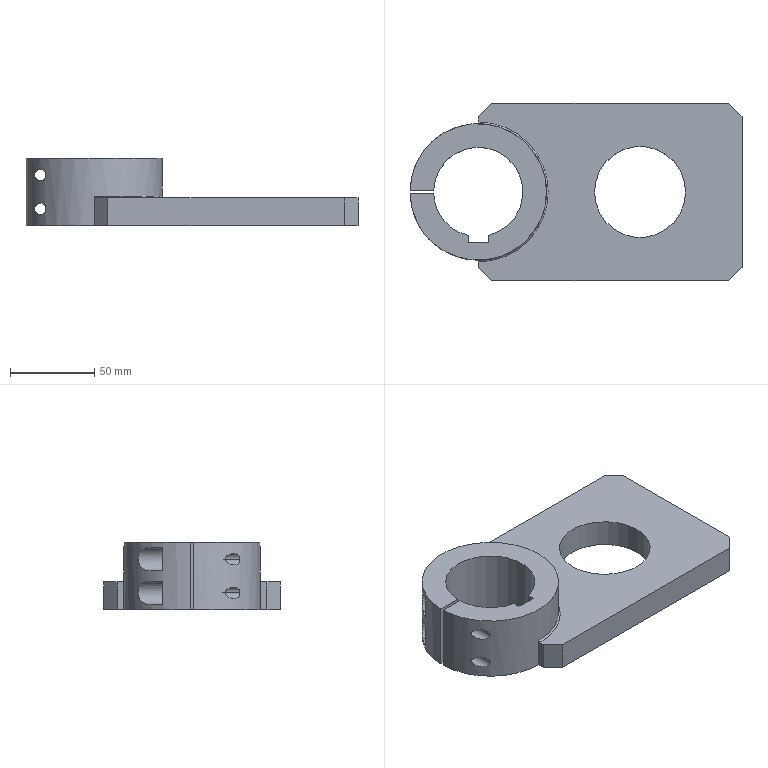Part | Creo | features CURVE 4, CUT 3, DATUM PLANE 3, CHAMFER 1, COORDINATE SYSTEM 1, PROTRUSION 1 | 1 solid | 42 faces | box 196.988 x 105 x 40 mm | volume 298699 mm3 | plane 26 | cylinder 15 | cone 1 | commonest cylinder face diameters 6.8 x8 14 x2 53 x2 54 x2 81 x1
STEP:
#1=CARTESIAN_POINT('',(0.,0.,0.));
#2=DIRECTION('',(0.,0.,1.));
#3=DIRECTION('',(1.,0.,0.));
#4=AXIS2_PLACEMENT_3D('',#1,#2,#3);
#5=CARTESIAN_POINT('',(-40.,44.5,0.));
#6=VERTEX_POINT('',#5);
#7=CARTESIAN_POINT('',(-40.,40.5,0.));
#8=VERTEX_POINT('',#7);
#9=CARTESIAN_POINT('',(-40.,44.5,0.));
#10=DIRECTION('',(0.,-1.,0.));
#11=VECTOR('',#10,4.);
#12=LINE('',#9,#11);
#13=EDGE_CURVE('',#6,#8,#12,.T.);
#14=ORIENTED_EDGE('',*,*,#13,.T.);
#15=CARTESIAN_POINT('',(-80.488,1.,0.));
#16=VERTEX_POINT('',#15);
#17=CARTESIAN_POINT('',(-40.,0.,0.));
#18=DIRECTION('',(0.,0.,1.));
#19=DIRECTION('',(0.,1.,0.));
#20=AXIS2_PLACEMENT_3D('',#17,#18,#19);
#21=CIRCLE('',#20,40.5);
#22=EDGE_CURVE('',#8,#16,#21,.T.);
#23=ORIENTED_EDGE('',*,*,#22,.T.);
#24=CARTESIAN_POINT('',(-66.481,1.,0.));
#25=VERTEX_POINT('',#24);
#26=CARTESIAN_POINT('',(-80.488,1.,0.));
#27=DIRECTION('',(1.,0.,0.));
#28=VECTOR('',#27,14.007);
#29=LINE('',#26,#28);
#30=EDGE_CURVE('',#16,#25,#29,.T.);
#31=ORIENTED_EDGE('',*,*,#30,.T.);
#32=CARTESIAN_POINT('',(-34.,-25.812,0.));
#33=VERTEX_POINT('',#32);
#34=CARTESIAN_POINT('',(-40.,0.,0.));
#35=DIRECTION('',(0.,0.,-1.));
#36=DIRECTION('',(-0.9993,0.03774,0.));
#37=AXIS2_PLACEMENT_3D('',#34,#35,#36);
#38=CIRCLE('',#37,26.5);
#39=EDGE_CURVE('',#25,#33,#38,.T.);
#40=ORIENTED_EDGE('',*,*,#39,.T.);
#41=CARTESIAN_POINT('',(-34.,-30.,0.));
#42=VERTEX_POINT('',#41);
#43=CARTESIAN_POINT('',(-34.,-25.812,0.));
#44=DIRECTION('',(0.,-1.,0.));
#45=VECTOR('',#44,4.188);
#46=LINE('',#43,#45);
#47=EDGE_CURVE('',#33,#42,#46,.T.);
#48=ORIENTED_EDGE('',*,*,#47,.T.);
#49=CARTESIAN_POINT('',(-40.,-30.,0.));
#50=VERTEX_POINT('',#49);
#51=CARTESIAN_POINT('',(-34.,-30.,0.));
#52=DIRECTION('',(-1.,0.,0.));
#53=VECTOR('',#52,6.);
#54=LINE('',#51,#53);
#55=EDGE_CURVE('',#42,#50,#54,.T.);
#56=ORIENTED_EDGE('',*,*,#55,.T.);
#57=CARTESIAN_POINT('',(-46.,-30.,0.));
#58=VERTEX_POINT('',#57);
#59=CARTESIAN_POINT('',(-40.,-30.,0.));
#60=DIRECTION('',(-1.,0.,0.));
#61=VECTOR('',#60,6.);
#62=LINE('',#59,#61);
#63=EDGE_CURVE('',#50,#58,#62,.T.);
#64=ORIENTED_EDGE('',*,*,#63,.T.);
#65=CARTESIAN_POINT('',(-46.,-25.812,0.));
#66=VERTEX_POINT('',#65);
#67=CARTESIAN_POINT('',(-46.,-30.,0.));
#68=DIRECTION('',(0.,1.,0.));
#69=VECTOR('',#68,4.188);
#70=LINE('',#67,#69);
#71=EDGE_CURVE('',#58,#66,#70,.T.);
#72=ORIENTED_EDGE('',*,*,#71,.T.);
#73=CARTESIAN_POINT('',(-66.481,-1.,0.));
#74=VERTEX_POINT('',#73);
#75=CARTESIAN_POINT('',(-40.,0.,0.));
#76=DIRECTION('',(0.,0.,-1.));
#77=DIRECTION('',(-0.2264,-0.974,0.));
#78=AXIS2_PLACEMENT_3D('',#75,#76,#77);
#79=CIRCLE('',#78,26.5);
#80=EDGE_CURVE('',#66,#74,#79,.T.);
#81=ORIENTED_EDGE('',*,*,#80,.T.);
#82=CARTESIAN_POINT('',(-80.488,-1.,0.));
#83=VERTEX_POINT('',#82);
#84=CARTESIAN_POINT('',(-66.481,-1.,0.));
#85=DIRECTION('',(-1.,0.,0.));
#86=VECTOR('',#85,14.007);
#87=LINE('',#84,#86);
#88=EDGE_CURVE('',#74,#83,#87,.T.);
#89=ORIENTED_EDGE('',*,*,#88,.T.);
#90=CARTESIAN_POINT('',(-40.,-40.5,0.));
#91=VERTEX_POINT('',#90);
#92=CARTESIAN_POINT('',(-40.,0.,0.));
#93=DIRECTION('',(0.,0.,1.));
#94=DIRECTION('',(-0.9997,-0.02469,0.));
#95=AXIS2_PLACEMENT_3D('',#92,#93,#94);
#96=CIRCLE('',#95,40.5);
#97=EDGE_CURVE('',#83,#91,#96,.T.);
#98=ORIENTED_EDGE('',*,*,#97,.T.);
#99=CARTESIAN_POINT('',(-40.,-44.5,0.));
#100=VERTEX_POINT('',#99);
#101=CARTESIAN_POINT('',(-40.,-40.5,0.));
#102=DIRECTION('',(0.,-1.,0.));
#103=VECTOR('',#102,4.);
#104=LINE('',#101,#103);
#105=EDGE_CURVE('',#91,#100,#104,.T.);
#106=ORIENTED_EDGE('',*,*,#105,.T.);
#107=CARTESIAN_POINT('',(-32.,-52.5,0.));
#108=VERTEX_POINT('',#107);
#109=CARTESIAN_POINT('',(-40.,-44.5,0.));
#110=DIRECTION('',(0.7071,-0.7071,0.));
#111=VECTOR('',#110,11.314);
#112=LINE('',#109,#111);
#113=EDGE_CURVE('',#100,#108,#112,.T.);
#114=ORIENTED_EDGE('',*,*,#113,.T.);
#115=CARTESIAN_POINT('',(108.5,-52.5,0.));
#116=VERTEX_POINT('',#115);
#117=CARTESIAN_POINT('',(-32.,-52.5,0.));
#118=DIRECTION('',(1.,0.,0.));
#119=VECTOR('',#118,140.5);
#120=LINE('',#117,#119);
#121=EDGE_CURVE('',#108,#116,#120,.T.);
#122=ORIENTED_EDGE('',*,*,#121,.T.);
#123=CARTESIAN_POINT('',(116.5,-44.5,0.));
#124=VERTEX_POINT('',#123);
#125=CARTESIAN_POINT('',(108.5,-52.5,0.));
#126=DIRECTION('',(0.7071,0.7071,0.));
#127=VECTOR('',#126,11.314);
#128=LINE('',#125,#127);
#129=EDGE_CURVE('',#116,#124,#128,.T.);
#130=ORIENTED_EDGE('',*,*,#129,.T.);
#131=CARTESIAN_POINT('',(116.5,44.5,0.));
#132=VERTEX_POINT('',#131);
#133=CARTESIAN_POINT('',(116.5,-44.5,0.));
#134=DIRECTION('',(0.,1.,0.));
#135=VECTOR('',#134,89.);
#136=LINE('',#133,#135);
#137=EDGE_CURVE('',#124,#132,#136,.T.);
#138=ORIENTED_EDGE('',*,*,#137,.T.);
#139=CARTESIAN_POINT('',(108.5,52.5,0.));
#140=VERTEX_POINT('',#139);
#141=CARTESIAN_POINT('',(116.5,44.5,0.));
#142=DIRECTION('',(-0.7071,0.7071,0.));
#143=VECTOR('',#142,11.314);
#144=LINE('',#141,#143);
#145=EDGE_CURVE('',#132,#140,#144,.T.);
#146=ORIENTED_EDGE('',*,*,#145,.T.);
#147=CARTESIAN_POINT('',(-32.,52.5,0.));
#148=VERTEX_POINT('',#147);
#149=CARTESIAN_POINT('',(108.5,52.5,0.));
#150=DIRECTION('',(-1.,0.,0.));
#151=VECTOR('',#150,140.5);
#152=LINE('',#149,#151);
#153=EDGE_CURVE('',#140,#148,#152,.T.);
#154=ORIENTED_EDGE('',*,*,#153,.T.);
#155=CARTESIAN_POINT('',(-32.,52.5,0.));
#156=DIRECTION('',(-0.7071,-0.7071,0.));
#157=VECTOR('',#156,11.314);
#158=LINE('',#155,#157);
#159=EDGE_CURVE('',#148,#6,#158,.T.);
#160=ORIENTED_EDGE('',*,*,#159,.T.);
#161=EDGE_LOOP('',(#14,#23,#31,#40,#48,#56,#64,#72,#81,#89,#98,#106,#114,#122,#130,#138,#146,#154,#160));
#162=FACE_OUTER_BOUND('',#161,.F.);
#163=CARTESIAN_POINT('',(83.,0.,0.));
#164=VERTEX_POINT('',#163);
#165=CARTESIAN_POINT('',(29.,0.,0.));
#166=VERTEX_POINT('',#165);
#167=CARTESIAN_POINT('',(56.,0.,0.));
#168=DIRECTION('',(0.,0.,-1.));
#169=DIRECTION('',(1.,0.,0.));
#170=AXIS2_PLACEMENT_3D('',#167,#168,#169);
#171=CIRCLE('',#170,27.);
#172=EDGE_CURVE('',#164,#166,#171,.T.);
#173=ORIENTED_EDGE('',*,*,#172,.T.);
#174=CARTESIAN_POINT('',(56.,0.,0.));
#175=DIRECTION('',(0.,0.,-1.));
#176=DIRECTION('',(-1.,0.,0.));
#177=AXIS2_PLACEMENT_3D('',#174,#175,#176);
#178=CIRCLE('',#177,27.);
#179=EDGE_CURVE('',#166,#164,#178,.T.);
#180=ORIENTED_EDGE('',*,*,#179,.T.);
#181=EDGE_LOOP('',(#173,#180));
#182=FACE_BOUND('',#181,.F.);
#183=CARTESIAN_POINT('',(0.,0.,0.));
#184=DIRECTION('',(0.,0.,1.));
#185=DIRECTION('',(1.,0.,0.));
#186=AXIS2_PLACEMENT_3D('',#183,#184,#185);
#187=PLANE('',#186);
#188=ADVANCED_FACE('',(#162,#182),#187,.F.);
#189=CARTESIAN_POINT('',(29.,0.,16.5));
#190=VERTEX_POINT('',#189);
#191=CARTESIAN_POINT('',(83.,0.,16.5));
#192=VERTEX_POINT('',#191);
#193=CARTESIAN_POINT('',(56.,0.,16.5));
#194=DIRECTION('',(0.,0.,1.));
#195=DIRECTION('',(-1.,0.,0.));
#196=AXIS2_PLACEMENT_3D('',#193,#194,#195);
#197=CIRCLE('',#196,27.);
#198=EDGE_CURVE('',#190,#192,#197,.T.);
#199=ORIENTED_EDGE('',*,*,#198,.F.);
#200=CARTESIAN_POINT('',(29.,0.,0.));
#201=DIRECTION('',(0.,0.,1.));
#202=VECTOR('',#201,16.5);
#203=LINE('',#200,#202);
#204=EDGE_CURVE('',#166,#190,#203,.T.);
#205=ORIENTED_EDGE('',*,*,#204,.F.);
#206=ORIENTED_EDGE('',*,*,#172,.F.);
#207=CARTESIAN_POINT('',(83.,0.,0.));
#208=DIRECTION('',(0.,0.,1.));
#209=VECTOR('',#208,16.5);
#210=LINE('',#207,#209);
#211=EDGE_CURVE('',#164,#192,#210,.T.);
#212=ORIENTED_EDGE('',*,*,#211,.T.);
#213=EDGE_LOOP('',(#199,#205,#206,#212));
#214=FACE_OUTER_BOUND('',#213,.F.);
#215=CARTESIAN_POINT('',(56.,0.,0.));
#216=DIRECTION('',(0.,0.,1.));
#217=DIRECTION('',(1.,0.,0.));
#218=AXIS2_PLACEMENT_3D('',#215,#216,#217);
#219=CYLINDRICAL_SURFACE('',#218,27.);
#220=ADVANCED_FACE('',(#214),#219,.F.);
#221=CARTESIAN_POINT('',(-40.,41.5,16.5));
#222=VERTEX_POINT('',#221);
#223=CARTESIAN_POINT('',(-40.,-41.5,16.5));
#224=VERTEX_POINT('',#223);
#225=CARTESIAN_POINT('',(-40.,0.000000008,16.5));
#226=DIRECTION('',(0.,0.,-1.));
#227=DIRECTION('',(0.,1.,0.));
#228=AXIS2_PLACEMENT_3D('',#225,#226,#227);
#229=CIRCLE('',#228,41.5);
#230=EDGE_CURVE('',#222,#224,#229,.T.);
#231=ORIENTED_EDGE('',*,*,#230,.F.);
#232=CARTESIAN_POINT('',(-40.,44.5,16.5));
#233=VERTEX_POINT('',#232);
#234=CARTESIAN_POINT('',(-40.,44.5,16.5));
#235=DIRECTION('',(0.,-1.,0.000000001));
#236=VECTOR('',#235,3.);
#237=LINE('',#234,#236);
#238=EDGE_CURVE('',#233,#222,#237,.T.);
#239=ORIENTED_EDGE('',*,*,#238,.F.);
#240=CARTESIAN_POINT('',(-32.,52.5,16.5));
#241=VERTEX_POINT('',#240);
#242=CARTESIAN_POINT('',(-32.,52.5,16.5));
#243=DIRECTION('',(-0.7071,-0.7071,0.));
#244=VECTOR('',#243,11.314);
#245=LINE('',#242,#244);
#246=EDGE_CURVE('',#241,#233,#245,.T.);
#247=ORIENTED_EDGE('',*,*,#246,.F.);
#248=CARTESIAN_POINT('',(108.5,52.5,16.5));
#249=VERTEX_POINT('',#248);
#250=CARTESIAN_POINT('',(108.5,52.5,16.5));
#251=DIRECTION('',(-1.,0.,0.));
#252=VECTOR('',#251,140.5);
#253=LINE('',#250,#252);
#254=EDGE_CURVE('',#249,#241,#253,.T.);
#255=ORIENTED_EDGE('',*,*,#254,.F.);
#256=CARTESIAN_POINT('',(116.5,44.5,16.5));
#257=VERTEX_POINT('',#256);
#258=CARTESIAN_POINT('',(116.5,44.5,16.5));
#259=DIRECTION('',(-0.7071,0.7071,0.));
#260=VECTOR('',#259,11.314);
#261=LINE('',#258,#260);
#262=EDGE_CURVE('',#257,#249,#261,.T.);
#263=ORIENTED_EDGE('',*,*,#262,.F.);
#264=CARTESIAN_POINT('',(116.5,-44.5,16.5));
#265=VERTEX_POINT('',#264);
#266=CARTESIAN_POINT('',(116.5,-44.5,16.5));
#267=DIRECTION('',(0.,1.,0.));
#268=VECTOR('',#267,89.);
#269=LINE('',#266,#268);
#270=EDGE_CURVE('',#265,#257,#269,.T.);
#271=ORIENTED_EDGE('',*,*,#270,.F.);
#272=CARTESIAN_POINT('',(108.5,-52.5,16.5));
#273=VERTEX_POINT('',#272);
#274=CARTESIAN_POINT('',(108.5,-52.5,16.5));
#275=DIRECTION('',(0.7071,0.7071,0.));
#276=VECTOR('',#275,11.314);
#277=LINE('',#274,#276);
#278=EDGE_CURVE('',#273,#265,#277,.T.);
#279=ORIENTED_EDGE('',*,*,#278,.F.);
#280=CARTESIAN_POINT('',(-32.,-52.5,16.5));
#281=VERTEX_POINT('',#280);
#282=CARTESIAN_POINT('',(-32.,-52.5,16.5));
#283=DIRECTION('',(1.,0.,0.));
#284=VECTOR('',#283,140.5);
#285=LINE('',#282,#284);
#286=EDGE_CURVE('',#281,#273,#285,.T.);
#287=ORIENTED_EDGE('',*,*,#286,.F.);
#288=CARTESIAN_POINT('',(-40.,-44.5,16.5));
#289=VERTEX_POINT('',#288);
#290=CARTESIAN_POINT('',(-40.,-44.5,16.5));
#291=DIRECTION('',(0.7071,-0.7071,0.));
#292=VECTOR('',#291,11.314);
#293=LINE('',#290,#292);
#294=EDGE_CURVE('',#289,#281,#293,.T.);
#295=ORIENTED_EDGE('',*,*,#294,.F.);
#296=CARTESIAN_POINT('',(-40.,-41.5,16.5));
#297=DIRECTION('',(0.,-1.,0.));
#298=VECTOR('',#297,3.);
#299=LINE('',#296,#298);
#300=EDGE_CURVE('',#224,#289,#299,.T.);
#301=ORIENTED_EDGE('',*,*,#300,.F.);
#302=EDGE_LOOP('',(#231,#239,#247,#255,#263,#271,#279,#287,#295,#301));
#303=FACE_OUTER_BOUND('',#302,.F.);
#304=ORIENTED_EDGE('',*,*,#198,.T.);
#305=CARTESIAN_POINT('',(56.,0.,16.5));
#306=DIRECTION('',(0.,0.,1.));
#307=DIRECTION('',(1.,0.,0.));
#308=AXIS2_PLACEMENT_3D('',#305,#306,#307);
#309=CIRCLE('',#308,27.);
#310=EDGE_CURVE('',#192,#190,#309,.T.);
#311=ORIENTED_EDGE('',*,*,#310,.T.);
#312=EDGE_LOOP('',(#304,#311));
#313=FACE_BOUND('',#312,.F.);
#314=CARTESIAN_POINT('',(0.,0.,16.5));
#315=DIRECTION('',(0.,0.,1.));
#316=DIRECTION('',(1.,0.,0.));
#317=AXIS2_PLACEMENT_3D('',#314,#315,#316);
#318=PLANE('',#317);
#319=ADVANCED_FACE('',(#303,#313),#318,.T.);
#320=ORIENTED_EDGE('',*,*,#310,.F.);
#321=ORIENTED_EDGE('',*,*,#211,.F.);
#322=ORIENTED_EDGE('',*,*,#179,.F.);
#323=ORIENTED_EDGE('',*,*,#204,.T.);
#324=EDGE_LOOP('',(#320,#321,#322,#323));
#325=FACE_OUTER_BOUND('',#324,.F.);
#326=CARTESIAN_POINT('',(56.,0.,0.));
#327=DIRECTION('',(0.,0.,1.));
#328=DIRECTION('',(1.,0.,0.));
#329=AXIS2_PLACEMENT_3D('',#326,#327,#328);
#330=CYLINDRICAL_SURFACE('',#329,27.);
#331=ADVANCED_FACE('',(#325),#330,.F.);
#332=CARTESIAN_POINT('',(-40.,-40.5,17.5));
#333=VERTEX_POINT('',#332);
#334=CARTESIAN_POINT('',(-40.,40.5,17.5));
#335=VERTEX_POINT('',#334);
#336=CARTESIAN_POINT('',(-40.,0.000000008,17.5));
#337=DIRECTION('',(0.,0.,1.));
#338=DIRECTION('',(0.,-1.,0.));
#339=AXIS2_PLACEMENT_3D('',#336,#337,#338);
#340=CIRCLE('',#339,40.5);
#341=EDGE_CURVE('',#333,#335,#340,.T.);
#342=ORIENTED_EDGE('',*,*,#341,.T.);
#343=CARTESIAN_POINT('',(-40.,40.5,17.5));
#344=DIRECTION('',(0.,0.7071,-0.7071));
#345=VECTOR('',#344,1.414);
#346=LINE('',#343,#345);
#347=EDGE_CURVE('',#335,#222,#346,.T.);
#348=ORIENTED_EDGE('',*,*,#347,.T.);
#349=ORIENTED_EDGE('',*,*,#230,.T.);
#350=CARTESIAN_POINT('',(-40.,-41.5,16.5));
#351=DIRECTION('',(0.,0.7071,0.7071));
#352=VECTOR('',#351,1.414);
#353=LINE('',#350,#352);
#354=EDGE_CURVE('',#224,#333,#353,.T.);
#355=ORIENTED_EDGE('',*,*,#354,.T.);
#356=EDGE_LOOP('',(#342,#348,#349,#355));
#357=FACE_OUTER_BOUND('',#356,.F.);
#358=CARTESIAN_POINT('',(-40.,0.000000008,17.));
#359=DIRECTION('',(0.,0.,-1.));
#360=DIRECTION('',(0.,-1.,0.));
#361=AXIS2_PLACEMENT_3D('',#358,#359,#360);
#362=CONICAL_SURFACE('',#361,41.,45.);
#363=ADVANCED_FACE('',(#357),#362,.T.);
#364=ORIENTED_EDGE('',*,*,#341,.F.);
#365=CARTESIAN_POINT('',(-40.,-40.5,0.));
#366=DIRECTION('',(0.,0.,1.));
#367=VECTOR('',#366,17.5);
#368=LINE('',#365,#367);
#369=EDGE_CURVE('',#91,#333,#368,.T.);
#370=ORIENTED_EDGE('',*,*,#369,.F.);
#371=ORIENTED_EDGE('',*,*,#97,.F.);
#372=CARTESIAN_POINT('',(-80.488,-1.,40.));
#373=VERTEX_POINT('',#372);
#374=CARTESIAN_POINT('',(-80.488,-1.,0.));
#375=DIRECTION('',(0.,0.,1.));
#376=VECTOR('',#375,40.);
#377=LINE('',#374,#376);
#378=EDGE_CURVE('',#83,#373,#377,.T.);
#379=ORIENTED_EDGE('',*,*,#378,.T.);
#380=CARTESIAN_POINT('',(-80.488,1.,40.));
#381=VERTEX_POINT('',#380);
#382=CARTESIAN_POINT('',(-40.,0.,40.));
#383=DIRECTION('',(0.,0.,1.));
#384=DIRECTION('',(-0.9997,-0.02469,0.));
#385=AXIS2_PLACEMENT_3D('',#382,#383,#384);
#386=CIRCLE('',#385,40.5);
#387=EDGE_CURVE('',#373,#381,#386,.T.);
#388=ORIENTED_EDGE('',*,*,#387,.T.);
#389=CARTESIAN_POINT('',(-80.488,1.,0.));
#390=DIRECTION('',(0.,0.,1.));
#391=VECTOR('',#390,40.);
#392=LINE('',#389,#391);
#393=EDGE_CURVE('',#16,#381,#392,.T.);
#394=ORIENTED_EDGE('',*,*,#393,.F.);
#395=ORIENTED_EDGE('',*,*,#22,.F.);
#396=CARTESIAN_POINT('',(-40.,40.5,17.5));
#397=DIRECTION('',(0.,0.,-1.));
#398=VECTOR('',#397,17.5);
#399=LINE('',#396,#398);
#400=EDGE_CURVE('',#335,#8,#399,.T.);
#401=ORIENTED_EDGE('',*,*,#400,.F.);
#402=EDGE_LOOP('',(#364,#370,#371,#379,#388,#394,#395,#401));
#403=FACE_OUTER_BOUND('',#402,.F.);
#404=CARTESIAN_POINT('',(-68.923,-28.35,8.554));
#405=VERTEX_POINT('',#404);
#406=CARTESIAN_POINT('',(-68.923,-28.35,11.446));
#407=VERTEX_POINT('',#406);
#408=CARTESIAN_POINT('',(-68.923,-28.35,8.554));
#409=DIRECTION('',(0.,0.,1.));
#410=VECTOR('',#409,2.892);
#411=LINE('',#408,#410);
#412=EDGE_CURVE('',#405,#407,#411,.T.);
#413=ORIENTED_EDGE('',*,*,#412,.T.);
#414=CARTESIAN_POINT('',(-75.4,-19.675,10.));
#415=VERTEX_POINT('',#414);
#416=CARTESIAN_POINT('',(-75.4,-19.675,10.194));
#417=CARTESIAN_POINT('',(-75.368,-19.733,10.574));
#418=CARTESIAN_POINT('',(-75.223,-19.992,11.133));
#419=CARTESIAN_POINT('',(-74.989,-20.398,11.652));
#420=CARTESIAN_POINT('',(-74.679,-20.922,12.118));
#421=CARTESIAN_POINT('',(-74.297,-21.544,12.528));
#422=CARTESIAN_POINT('',(-73.838,-22.26,12.88));
#423=CARTESIAN_POINT('',(-73.311,-23.043,13.157));
#424=CARTESIAN_POINT('',(-72.705,-23.897,13.348));
#425=CARTESIAN_POINT('',(-72.034,-24.789,13.423));
#426=CARTESIAN_POINT('',(-71.32,-25.686,13.359));
#427=CARTESIAN_POINT('',(-70.573,-26.57,13.122));
#428=CARTESIAN_POINT('',(-69.869,-27.357,12.69));
#429=CARTESIAN_POINT('',(-69.31,-27.952,12.128));
#430=CARTESIAN_POINT('',(-69.035,-28.235,11.685));
#431=CARTESIAN_POINT('',(-68.923,-28.35,11.446));
#432=B_SPLINE_CURVE_WITH_KNOTS('',3,(#414,#416,#417,#418,#419,#420,#421,#422,#423,#424,#425,#426,#427,#428,#429,#430,#431),.UNSPECIFIED.,.F.,.F.,(4,1,1,1,1,1,1,1,1,1,1,1,1,1,4),(0.,0.07143,0.1429,0.2143,0.2857,0.3571,0.4286,0.5,0.5714,0.6429,0.7143,0.7857,0.8571,0.9286,1.),.UNSPECIFIED.);
#433=EDGE_CURVE('',#415,#407,#432,.T.);
#434=ORIENTED_EDGE('',*,*,#433,.F.);
#435=CARTESIAN_POINT('',(-68.923,-28.35,8.554));
#436=CARTESIAN_POINT('',(-69.044,-28.226,8.296));
#437=CARTESIAN_POINT('',(-69.345,-27.916,7.819));
#438=CARTESIAN_POINT('',(-69.987,-27.23,7.211));
#439=CARTESIAN_POINT('',(-70.781,-26.331,6.786));
#440=CARTESIAN_POINT('',(-71.589,-25.356,6.595));
#441=CARTESIAN_POINT('',(-72.34,-24.39,6.591));
#442=CARTESIAN_POINT('',(-73.025,-23.452,6.735));
#443=CARTESIAN_POINT('',(-73.627,-22.579,6.992));
#444=CARTESIAN_POINT('',(-74.14,-21.795,7.334));
#445=CARTESIAN_POINT('',(-74.579,-21.089,7.757));
#446=CARTESIAN_POINT('',(-74.931,-20.499,8.243));
#447=CARTESIAN_POINT('',(-75.192,-20.045,8.778));
#448=CARTESIAN_POINT('',(-75.361,-19.745,9.375));
#449=CARTESIAN_POINT('',(-75.4,-19.675,9.788));
#450=CARTESIAN_POINT('',(-75.4,-19.675,10.));
#451=B_SPLINE_CURVE_WITH_KNOTS('',3,(#435,#436,#437,#438,#439,#440,#441,#442,#443,#444,#445,#446,#447,#448,#449,#450),.UNSPECIFIED.,.F.,.F.,(4,1,1,1,1,1,1,1,1,1,1,1,1,4),(0.,0.07692,0.1538,0.2308,0.3077,0.3846,0.4615,0.5385,0.6154,0.6923,0.7692,0.8462,0.9231,1.),.UNSPECIFIED.);
#452=EDGE_CURVE('',#405,#415,#451,.T.);
#453=ORIENTED_EDGE('',*,*,#452,.F.);
#454=EDGE_LOOP('',(#413,#434,#453));
#455=FACE_BOUND('',#454,.F.);
#456=CARTESIAN_POINT('',(-68.923,-28.35,28.554));
#457=VERTEX_POINT('',#456);
#458=CARTESIAN_POINT('',(-68.923,-28.35,31.446));
#459=VERTEX_POINT('',#458);
#460=CARTESIAN_POINT('',(-68.923,-28.35,28.554));
#461=DIRECTION('',(0.,0.,1.));
#462=VECTOR('',#461,2.892);
#463=LINE('',#460,#462);
#464=EDGE_CURVE('',#457,#459,#463,.T.);
#465=ORIENTED_EDGE('',*,*,#464,.T.);
#466=CARTESIAN_POINT('',(-75.4,-19.675,30.));
#467=VERTEX_POINT('',#466);
#468=CARTESIAN_POINT('',(-75.4,-19.675,30.194));
#469=CARTESIAN_POINT('',(-75.368,-19.733,30.574));
#470=CARTESIAN_POINT('',(-75.223,-19.992,31.133));
#471=CARTESIAN_POINT('',(-74.989,-20.398,31.652));
#472=CARTESIAN_POINT('',(-74.679,-20.922,32.118));
#473=CARTESIAN_POINT('',(-74.297,-21.544,32.528));
#474=CARTESIAN_POINT('',(-73.838,-22.26,32.88));
#475=CARTESIAN_POINT('',(-73.311,-23.043,33.157));
#476=CARTESIAN_POINT('',(-72.705,-23.897,33.348));
#477=CARTESIAN_POINT('',(-72.034,-24.789,33.423));
#478=CARTESIAN_POINT('',(-71.32,-25.686,33.359));
#479=CARTESIAN_POINT('',(-70.573,-26.57,33.122));
#480=CARTESIAN_POINT('',(-69.869,-27.357,32.69));
#481=CARTESIAN_POINT('',(-69.31,-27.952,32.128));
#482=CARTESIAN_POINT('',(-69.035,-28.235,31.685));
#483=CARTESIAN_POINT('',(-68.923,-28.35,31.446));
#484=B_SPLINE_CURVE_WITH_KNOTS('',3,(#466,#468,#469,#470,#471,#472,#473,#474,#475,#476,#477,#478,#479,#480,#481,#482,#483),.UNSPECIFIED.,.F.,.F.,(4,1,1,1,1,1,1,1,1,1,1,1,1,1,4),(0.,0.07143,0.1429,0.2143,0.2857,0.3571,0.4286,0.5,0.5714,0.6429,0.7143,0.7857,0.8571,0.9286,1.),.UNSPECIFIED.);
#485=EDGE_CURVE('',#467,#459,#484,.T.);
#486=ORIENTED_EDGE('',*,*,#485,.F.);
#487=CARTESIAN_POINT('',(-68.923,-28.35,28.554));
#488=CARTESIAN_POINT('',(-69.044,-28.226,28.296));
#489=CARTESIAN_POINT('',(-69.345,-27.916,27.819));
#490=CARTESIAN_POINT('',(-69.987,-27.23,27.211));
#491=CARTESIAN_POINT('',(-70.781,-26.331,26.786));
#492=CARTESIAN_POINT('',(-71.589,-25.356,26.595));
#493=CARTESIAN_POINT('',(-72.34,-24.39,26.591));
#494=CARTESIAN_POINT('',(-73.025,-23.452,26.735));
#495=CARTESIAN_POINT('',(-73.627,-22.579,26.992));
#496=CARTESIAN_POINT('',(-74.14,-21.795,27.334));
#497=CARTESIAN_POINT('',(-74.579,-21.089,27.757));
#498=CARTESIAN_POINT('',(-74.931,-20.499,28.243));
#499=CARTESIAN_POINT('',(-75.192,-20.045,28.778));
#500=CARTESIAN_POINT('',(-75.361,-19.745,29.375));
#501=CARTESIAN_POINT('',(-75.4,-19.675,29.788));
#502=CARTESIAN_POINT('',(-75.4,-19.675,30.));
#503=B_SPLINE_CURVE_WITH_KNOTS('',3,(#487,#488,#489,#490,#491,#492,#493,#494,#495,#496,#497,#498,#499,#500,#501,#502),.UNSPECIFIED.,.F.,.F.,(4,1,1,1,1,1,1,1,1,1,1,1,1,4),(0.,0.07692,0.1538,0.2308,0.3077,0.3846,0.4615,0.5385,0.6154,0.6923,0.7692,0.8462,0.9231,1.),.UNSPECIFIED.);
#504=EDGE_CURVE('',#457,#467,#503,.T.);
#505=ORIENTED_EDGE('',*,*,#504,.F.);
#506=EDGE_LOOP('',(#465,#486,#505));
#507=FACE_BOUND('',#506,.F.);
#508=CARTESIAN_POINT('',(-76.524,17.5,3.));
#509=VERTEX_POINT('',#508);
#510=CARTESIAN_POINT('',(-76.524,17.5,17.));
#511=VERTEX_POINT('',#510);
#512=CARTESIAN_POINT('',(-76.524,17.5,3.));
#513=DIRECTION('',(0.,0.,1.));
#514=VECTOR('',#513,14.);
#515=LINE('',#512,#514);
#516=EDGE_CURVE('',#509,#511,#515,.T.);
#517=ORIENTED_EDGE('',*,*,#516,.T.);
#518=CARTESIAN_POINT('',(-72.,24.824,17.));
#519=VERTEX_POINT('',#518);
#520=CARTESIAN_POINT('',(-40.,0.,17.));
#521=DIRECTION('',(0.,0.,1.));
#522=DIRECTION('',(-0.7901,0.6129,0.));
#523=AXIS2_PLACEMENT_3D('',#520,#521,#522);
#524=CIRCLE('',#523,40.5);
#525=EDGE_CURVE('',#519,#511,#524,.T.);
#526=ORIENTED_EDGE('',*,*,#525,.F.);
#527=CARTESIAN_POINT('',(-72.,24.824,3.));
#528=VERTEX_POINT('',#527);
#529=CARTESIAN_POINT('',(-71.732,25.17,3.));
#530=CARTESIAN_POINT('',(-71.187,25.849,3.031));
#531=CARTESIAN_POINT('',(-70.34,26.839,3.181));
#532=CARTESIAN_POINT('',(-69.473,27.787,3.45));
#533=CARTESIAN_POINT('',(-68.599,28.685,3.855));
#534=CARTESIAN_POINT('',(-67.74,29.516,4.412));
#535=CARTESIAN_POINT('',(-66.929,30.256,5.131));
#536=CARTESIAN_POINT('',(-66.195,30.893,6.028));
#537=CARTESIAN_POINT('',(-65.577,31.405,7.117));
#538=CARTESIAN_POINT('',(-65.132,31.76,8.417));
#539=CARTESIAN_POINT('',(-64.952,31.901,9.857));
#540=CARTESIAN_POINT('',(-65.07,31.809,11.283));
#541=CARTESIAN_POINT('',(-65.464,31.495,12.623));
#542=CARTESIAN_POINT('',(-66.046,31.018,13.748));
#543=CARTESIAN_POINT('',(-66.774,30.394,14.705));
#544=CARTESIAN_POINT('',(-67.593,29.653,15.476));
#545=CARTESIAN_POINT('',(-68.484,28.8,16.083));
#546=CARTESIAN_POINT('',(-69.391,27.875,16.52));
#547=CARTESIAN_POINT('',(-70.292,26.894,16.809));
#548=CARTESIAN_POINT('',(-71.168,25.873,16.968));
#549=CARTESIAN_POINT('',(-71.726,25.177,17.));
#550=CARTESIAN_POINT('',(-72.,24.824,17.));
#551=B_SPLINE_CURVE_WITH_KNOTS('',3,(#527,#529,#530,#531,#532,#533,#534,#535,#536,#537,#538,#539,#540,#541,#542,#543,#544,#545,#546,#547,#548,#549,#550),.UNSPECIFIED.,.F.,.F.,(4,1,1,1,1,1,1,1,1,1,1,1,1,1,1,1,1,1,1,1,4),(0.,0.05,0.1,0.15,0.2,0.25,0.3,0.35,0.4,0.45,0.5,0.55,0.6,0.65,0.7,0.75,0.8,0.85,0.9,0.95,1.),.UNSPECIFIED.);
#552=EDGE_CURVE('',#528,#519,#551,.T.);
#553=ORIENTED_EDGE('',*,*,#552,.F.);
#554=CARTESIAN_POINT('',(-40.,0.,3.));
#555=DIRECTION('',(0.,0.,1.));
#556=DIRECTION('',(-0.7901,0.6129,0.));
#557=AXIS2_PLACEMENT_3D('',#554,#555,#556);
#558=CIRCLE('',#557,40.5);
#559=EDGE_CURVE('',#528,#509,#558,.T.);
#560=ORIENTED_EDGE('',*,*,#559,.T.);
#561=EDGE_LOOP('',(#517,#526,#553,#560));
#562=FACE_BOUND('',#561,.F.);
#563=CARTESIAN_POINT('',(-76.524,17.5,23.));
#564=VERTEX_POINT('',#563);
#565=CARTESIAN_POINT('',(-76.524,17.5,37.));
#566=VERTEX_POINT('',#565);
#567=CARTESIAN_POINT('',(-76.524,17.5,23.));
#568=DIRECTION('',(0.,0.,1.));
#569=VECTOR('',#568,14.);
#570=LINE('',#567,#569);
#571=EDGE_CURVE('',#564,#566,#570,.T.);
#572=ORIENTED_EDGE('',*,*,#571,.T.);
#573=CARTESIAN_POINT('',(-72.,24.824,37.));
#574=VERTEX_POINT('',#573);
#575=CARTESIAN_POINT('',(-40.,0.,37.));
#576=DIRECTION('',(0.,0.,1.));
#577=DIRECTION('',(-0.7901,0.6129,0.));
#578=AXIS2_PLACEMENT_3D('',#575,#576,#577);
#579=CIRCLE('',#578,40.5);
#580=EDGE_CURVE('',#574,#566,#579,.T.);
#581=ORIENTED_EDGE('',*,*,#580,.F.);
#582=CARTESIAN_POINT('',(-72.,24.824,23.));
#583=VERTEX_POINT('',#582);
#584=CARTESIAN_POINT('',(-71.732,25.17,23.));
#585=CARTESIAN_POINT('',(-71.187,25.849,23.031));
#586=CARTESIAN_POINT('',(-70.34,26.839,23.181));
#587=CARTESIAN_POINT('',(-69.473,27.787,23.45));
#588=CARTESIAN_POINT('',(-68.599,28.685,23.855));
#589=CARTESIAN_POINT('',(-67.74,29.516,24.412));
#590=CARTESIAN_POINT('',(-66.929,30.256,25.131));
#591=CARTESIAN_POINT('',(-66.195,30.893,26.028));
#592=CARTESIAN_POINT('',(-65.577,31.405,27.117));
#593=CARTESIAN_POINT('',(-65.132,31.76,28.417));
#594=CARTESIAN_POINT('',(-64.952,31.901,29.857));
#595=CARTESIAN_POINT('',(-65.07,31.809,31.283));
#596=CARTESIAN_POINT('',(-65.464,31.495,32.623));
#597=CARTESIAN_POINT('',(-66.046,31.018,33.748));
#598=CARTESIAN_POINT('',(-66.774,30.394,34.705));
#599=CARTESIAN_POINT('',(-67.593,29.653,35.476));
#600=CARTESIAN_POINT('',(-68.484,28.8,36.083));
#601=CARTESIAN_POINT('',(-69.391,27.875,36.52));
#602=CARTESIAN_POINT('',(-70.292,26.894,36.809));
#603=CARTESIAN_POINT('',(-71.168,25.873,36.968));
#604=CARTESIAN_POINT('',(-71.726,25.177,37.));
#605=CARTESIAN_POINT('',(-72.,24.824,37.));
#606=B_SPLINE_CURVE_WITH_KNOTS('',3,(#582,#584,#585,#586,#587,#588,#589,#590,#591,#592,#593,#594,#595,#596,#597,#598,#599,#600,#601,#602,#603,#604,#605),.UNSPECIFIED.,.F.,.F.,(4,1,1,1,1,1,1,1,1,1,1,1,1,1,1,1,1,1,1,1,4),(0.,0.05,0.1,0.15,0.2,0.25,0.3,0.35,0.4,0.45,0.5,0.55,0.6,0.65,0.7,0.75,0.8,0.85,0.9,0.95,1.),.UNSPECIFIED.);
#607=EDGE_CURVE('',#583,#574,#606,.T.);
#608=ORIENTED_EDGE('',*,*,#607,.F.);
#609=CARTESIAN_POINT('',(-40.,0.,23.));
#610=DIRECTION('',(0.,0.,1.));
#611=DIRECTION('',(-0.7901,0.6129,0.));
#612=AXIS2_PLACEMENT_3D('',#609,#610,#611);
#613=CIRCLE('',#612,40.5);
#614=EDGE_CURVE('',#583,#564,#613,.T.);
#615=ORIENTED_EDGE('',*,*,#614,.T.);
#616=EDGE_LOOP('',(#572,#581,#608,#615));
#617=FACE_BOUND('',#616,.F.);
#618=CARTESIAN_POINT('',(-40.,0.,0.));
#619=DIRECTION('',(0.,0.,1.));
#620=DIRECTION('',(1.,0.,0.));
#621=AXIS2_PLACEMENT_3D('',#618,#619,#620);
#622=CYLINDRICAL_SURFACE('',#621,40.5);
#623=ADVANCED_FACE('',(#403,#455,#507,#562,#617),#622,.T.);
#624=ORIENTED_EDGE('',*,*,#369,.T.);
#625=ORIENTED_EDGE('',*,*,#354,.F.);
#626=ORIENTED_EDGE('',*,*,#300,.T.);
#627=CARTESIAN_POINT('',(-40.,-44.5,0.));
#628=DIRECTION('',(0.,0.,1.));
#629=VECTOR('',#628,16.5);
#630=LINE('',#627,#629);
#631=EDGE_CURVE('',#100,#289,#630,.T.);
#632=ORIENTED_EDGE('',*,*,#631,.F.);
#633=ORIENTED_EDGE('',*,*,#105,.F.);
#634=EDGE_LOOP('',(#624,#625,#626,#632,#633));
#635=FACE_OUTER_BOUND('',#634,.F.);
#636=CARTESIAN_POINT('',(-40.,-40.5,0.));
#637=DIRECTION('',(-1.,0.,0.));
#638=DIRECTION('',(0.,-1.,0.));
#639=AXIS2_PLACEMENT_3D('',#636,#637,#638);
#640=PLANE('',#639);
#641=ADVANCED_FACE('',(#635),#640,.T.);
#642=ORIENTED_EDGE('',*,*,#294,.T.);
#643=CARTESIAN_POINT('',(-32.,-52.5,0.));
#644=DIRECTION('',(0.,0.,1.));
#645=VECTOR('',#644,16.5);
#646=LINE('',#643,#645);
#647=EDGE_CURVE('',#108,#281,#646,.T.);
#648=ORIENTED_EDGE('',*,*,#647,.F.);
#649=ORIENTED_EDGE('',*,*,#113,.F.);
#650=ORIENTED_EDGE('',*,*,#631,.T.);
#651=EDGE_LOOP('',(#642,#648,#649,#650));
#652=FACE_OUTER_BOUND('',#651,.F.);
#653=CARTESIAN_POINT('',(-40.,-44.5,0.));
#654=DIRECTION('',(-0.7071,-0.7071,0.));
#655=DIRECTION('',(0.7071,-0.7071,0.));
#656=AXIS2_PLACEMENT_3D('',#653,#654,#655);
#657=PLANE('',#656);
#658=ADVANCED_FACE('',(#652),#657,.T.);
#659=ORIENTED_EDGE('',*,*,#286,.T.);
#660=CARTESIAN_POINT('',(108.5,-52.5,0.));
#661=DIRECTION('',(0.,0.,1.));
#662=VECTOR('',#661,16.5);
#663=LINE('',#660,#662);
#664=EDGE_CURVE('',#116,#273,#663,.T.);
#665=ORIENTED_EDGE('',*,*,#664,.F.);
#666=ORIENTED_EDGE('',*,*,#121,.F.);
#667=ORIENTED_EDGE('',*,*,#647,.T.);
#668=EDGE_LOOP('',(#659,#665,#666,#667));
#669=FACE_OUTER_BOUND('',#668,.F.);
#670=CARTESIAN_POINT('',(-32.,-52.5,0.));
#671=DIRECTION('',(0.,-1.,0.));
#672=DIRECTION('',(1.,0.,0.));
#673=AXIS2_PLACEMENT_3D('',#670,#671,#672);
#674=PLANE('',#673);
#675=ADVANCED_FACE('',(#669),#674,.T.);
#676=ORIENTED_EDGE('',*,*,#278,.T.);
#677=CARTESIAN_POINT('',(116.5,-44.5,0.));
#678=DIRECTION('',(0.,0.,1.));
#679=VECTOR('',#678,16.5);
#680=LINE('',#677,#679);
#681=EDGE_CURVE('',#124,#265,#680,.T.);
#682=ORIENTED_EDGE('',*,*,#681,.F.);
#683=ORIENTED_EDGE('',*,*,#129,.F.);
#684=ORIENTED_EDGE('',*,*,#664,.T.);
#685=EDGE_LOOP('',(#676,#682,#683,#684));
#686=FACE_OUTER_BOUND('',#685,.F.);
#687=CARTESIAN_POINT('',(108.5,-52.5,0.));
#688=DIRECTION('',(0.7071,-0.7071,0.));
#689=DIRECTION('',(0.7071,0.7071,0.));
#690=AXIS2_PLACEMENT_3D('',#687,#688,#689);
#691=PLANE('',#690);
#692=ADVANCED_FACE('',(#686),#691,.T.);
#693=ORIENTED_EDGE('',*,*,#270,.T.);
#694=CARTESIAN_POINT('',(116.5,44.5,0.));
#695=DIRECTION('',(0.,0.,1.));
#696=VECTOR('',#695,16.5);
#697=LINE('',#694,#696);
#698=EDGE_CURVE('',#132,#257,#697,.T.);
#699=ORIENTED_EDGE('',*,*,#698,.F.);
#700=ORIENTED_EDGE('',*,*,#137,.F.);
#701=ORIENTED_EDGE('',*,*,#681,.T.);
#702=EDGE_LOOP('',(#693,#699,#700,#701));
#703=FACE_OUTER_BOUND('',#702,.F.);
#704=CARTESIAN_POINT('',(116.5,-44.5,0.));
#705=DIRECTION('',(1.,0.,0.));
#706=DIRECTION('',(0.,1.,0.));
#707=AXIS2_PLACEMENT_3D('',#704,#705,#706);
#708=PLANE('',#707);
#709=ADVANCED_FACE('',(#703),#708,.T.);
#710=ORIENTED_EDGE('',*,*,#262,.T.);
#711=CARTESIAN_POINT('',(108.5,52.5,0.));
#712=DIRECTION('',(0.,0.,1.));
#713=VECTOR('',#712,16.5);
#714=LINE('',#711,#713);
#715=EDGE_CURVE('',#140,#249,#714,.T.);
#716=ORIENTED_EDGE('',*,*,#715,.F.);
#717=ORIENTED_EDGE('',*,*,#145,.F.);
#718=ORIENTED_EDGE('',*,*,#698,.T.);
#719=EDGE_LOOP('',(#710,#716,#717,#718));
#720=FACE_OUTER_BOUND('',#719,.F.);
#721=CARTESIAN_POINT('',(116.5,44.5,0.));
#722=DIRECTION('',(0.7071,0.7071,0.));
#723=DIRECTION('',(-0.7071,0.7071,0.));
#724=AXIS2_PLACEMENT_3D('',#721,#722,#723);
#725=PLANE('',#724);
#726=ADVANCED_FACE('',(#720),#725,.T.);
#727=ORIENTED_EDGE('',*,*,#254,.T.);
#728=CARTESIAN_POINT('',(-32.,52.5,0.));
#729=DIRECTION('',(0.,0.,1.));
#730=VECTOR('',#729,16.5);
#731=LINE('',#728,#730);
#732=EDGE_CURVE('',#148,#241,#731,.T.);
#733=ORIENTED_EDGE('',*,*,#732,.F.);
#734=ORIENTED_EDGE('',*,*,#153,.F.);
#735=ORIENTED_EDGE('',*,*,#715,.T.);
#736=EDGE_LOOP('',(#727,#733,#734,#735));
#737=FACE_OUTER_BOUND('',#736,.F.);
#738=CARTESIAN_POINT('',(108.5,52.5,0.));
#739=DIRECTION('',(0.,1.,0.));
#740=DIRECTION('',(-1.,0.,0.));
#741=AXIS2_PLACEMENT_3D('',#738,#739,#740);
#742=PLANE('',#741);
#743=ADVANCED_FACE('',(#737),#742,.T.);
#744=ORIENTED_EDGE('',*,*,#246,.T.);
#745=CARTESIAN_POINT('',(-40.,44.5,0.));
#746=DIRECTION('',(0.,0.,1.));
#747=VECTOR('',#746,16.5);
#748=LINE('',#745,#747);
#749=EDGE_CURVE('',#6,#233,#748,.T.);
#750=ORIENTED_EDGE('',*,*,#749,.F.);
#751=ORIENTED_EDGE('',*,*,#159,.F.);
#752=ORIENTED_EDGE('',*,*,#732,.T.);
#753=EDGE_LOOP('',(#744,#750,#751,#752));
#754=FACE_OUTER_BOUND('',#753,.F.);
#755=CARTESIAN_POINT('',(-32.,52.5,0.));
#756=DIRECTION('',(-0.7071,0.7071,0.));
#757=DIRECTION('',(-0.7071,-0.7071,0.));
#758=AXIS2_PLACEMENT_3D('',#755,#756,#757);
#759=PLANE('',#758);
#760=ADVANCED_FACE('',(#754),#759,.T.);
#761=ORIENTED_EDGE('',*,*,#238,.T.);
#762=ORIENTED_EDGE('',*,*,#347,.F.);
#763=ORIENTED_EDGE('',*,*,#400,.T.);
#764=ORIENTED_EDGE('',*,*,#13,.F.);
#765=ORIENTED_EDGE('',*,*,#749,.T.);
#766=EDGE_LOOP('',(#761,#762,#763,#764,#765));
#767=FACE_OUTER_BOUND('',#766,.F.);
#768=CARTESIAN_POINT('',(-40.,44.5,0.));
#769=DIRECTION('',(-1.,0.,0.));
#770=DIRECTION('',(0.,-1.,0.));
#771=AXIS2_PLACEMENT_3D('',#768,#769,#770);
#772=PLANE('',#771);
#773=ADVANCED_FACE('',(#767),#772,.T.);
#774=ORIENTED_EDGE('',*,*,#88,.F.);
#775=CARTESIAN_POINT('',(-66.481,-1.,40.));
#776=VERTEX_POINT('',#775);
#777=CARTESIAN_POINT('',(-66.481,-1.,0.));
#778=DIRECTION('',(0.,0.,1.));
#779=VECTOR('',#778,40.);
#780=LINE('',#777,#779);
#781=EDGE_CURVE('',#74,#776,#780,.T.);
#782=ORIENTED_EDGE('',*,*,#781,.T.);
#783=CARTESIAN_POINT('',(-66.481,-1.,40.));
#784=DIRECTION('',(-1.,0.,0.));
#785=VECTOR('',#784,14.007);
#786=LINE('',#783,#785);
#787=EDGE_CURVE('',#776,#373,#786,.T.);
#788=ORIENTED_EDGE('',*,*,#787,.T.);
#789=ORIENTED_EDGE('',*,*,#378,.F.);
#790=EDGE_LOOP('',(#774,#782,#788,#789));
#791=FACE_OUTER_BOUND('',#790,.F.);
#792=CARTESIAN_POINT('',(-75.4,-1.,30.));
#793=VERTEX_POINT('',#792);
#794=CARTESIAN_POINT('',(-68.6,-1.,30.));
#795=VERTEX_POINT('',#794);
#796=CARTESIAN_POINT('',(-72.,-1.,30.));
#797=DIRECTION('',(0.,1.,0.));
#798=DIRECTION('',(-1.,0.,0.));
#799=AXIS2_PLACEMENT_3D('',#796,#797,#798);
#800=CIRCLE('',#799,3.4);
#801=EDGE_CURVE('',#793,#795,#800,.T.);
#802=ORIENTED_EDGE('',*,*,#801,.T.);
#803=CARTESIAN_POINT('',(-72.,-1.,30.));
#804=DIRECTION('',(0.,1.,0.));
#805=DIRECTION('',(1.,0.,0.));
#806=AXIS2_PLACEMENT_3D('',#803,#804,#805);
#807=CIRCLE('',#806,3.4);
#808=EDGE_CURVE('',#795,#793,#807,.T.);
#809=ORIENTED_EDGE('',*,*,#808,.T.);
#810=EDGE_LOOP('',(#802,#809));
#811=FACE_BOUND('',#810,.F.);
#812=CARTESIAN_POINT('',(-75.4,-1.,10.));
#813=VERTEX_POINT('',#812);
#814=CARTESIAN_POINT('',(-68.6,-1.,10.));
#815=VERTEX_POINT('',#814);
#816=CARTESIAN_POINT('',(-72.,-1.,10.));
#817=DIRECTION('',(0.,1.,0.));
#818=DIRECTION('',(-1.,0.,0.));
#819=AXIS2_PLACEMENT_3D('',#816,#817,#818);
#820=CIRCLE('',#819,3.4);
#821=EDGE_CURVE('',#813,#815,#820,.T.);
#822=ORIENTED_EDGE('',*,*,#821,.T.);
#823=CARTESIAN_POINT('',(-72.,-1.,10.));
#824=DIRECTION('',(0.,1.,0.));
#825=DIRECTION('',(1.,0.,0.));
#826=AXIS2_PLACEMENT_3D('',#823,#824,#825);
#827=CIRCLE('',#826,3.4);
#828=EDGE_CURVE('',#815,#813,#827,.T.);
#829=ORIENTED_EDGE('',*,*,#828,.T.);
#830=EDGE_LOOP('',(#822,#829));
#831=FACE_BOUND('',#830,.F.);
#832=CARTESIAN_POINT('',(-66.481,-1.,0.));
#833=DIRECTION('',(0.,1.,0.));
#834=DIRECTION('',(-1.,0.,0.));
#835=AXIS2_PLACEMENT_3D('',#832,#833,#834);
#836=PLANE('',#835);
#837=ADVANCED_FACE('',(#791,#811,#831),#836,.T.);
#838=ORIENTED_EDGE('',*,*,#80,.F.);
#839=CARTESIAN_POINT('',(-46.,-25.812,40.));
#840=VERTEX_POINT('',#839);
#841=CARTESIAN_POINT('',(-46.,-25.812,0.));
#842=DIRECTION('',(0.,0.,1.));
#843=VECTOR('',#842,40.);
#844=LINE('',#841,#843);
#845=EDGE_CURVE('',#66,#840,#844,.T.);
#846=ORIENTED_EDGE('',*,*,#845,.T.);
#847=CARTESIAN_POINT('',(-40.,0.,40.));
#848=DIRECTION('',(0.,0.,-1.));
#849=DIRECTION('',(-0.2264,-0.974,0.));
#850=AXIS2_PLACEMENT_3D('',#847,#848,#849);
#851=CIRCLE('',#850,26.5);
#852=EDGE_CURVE('',#840,#776,#851,.T.);
#853=ORIENTED_EDGE('',*,*,#852,.T.);
#854=ORIENTED_EDGE('',*,*,#781,.F.);
#855=EDGE_LOOP('',(#838,#846,#853,#854));
#856=FACE_OUTER_BOUND('',#855,.F.);
#857=CARTESIAN_POINT('',(-40.,0.,0.));
#858=DIRECTION('',(0.,0.,1.));
#859=DIRECTION('',(1.,0.,0.));
#860=AXIS2_PLACEMENT_3D('',#857,#858,#859);
#861=CYLINDRICAL_SURFACE('',#860,26.5);
#862=ADVANCED_FACE('',(#856),#861,.F.);
#863=ORIENTED_EDGE('',*,*,#71,.F.);
#864=CARTESIAN_POINT('',(-46.,-30.,40.));
#865=VERTEX_POINT('',#864);
#866=CARTESIAN_POINT('',(-46.,-30.,0.));
#867=DIRECTION('',(0.,0.,1.));
#868=VECTOR('',#867,40.);
#869=LINE('',#866,#868);
#870=EDGE_CURVE('',#58,#865,#869,.T.);
#871=ORIENTED_EDGE('',*,*,#870,.T.);
#872=CARTESIAN_POINT('',(-46.,-30.,40.));
#873=DIRECTION('',(0.,1.,0.));
#874=VECTOR('',#873,4.188);
#875=LINE('',#872,#874);
#876=EDGE_CURVE('',#865,#840,#875,.T.);
#877=ORIENTED_EDGE('',*,*,#876,.T.);
#878=ORIENTED_EDGE('',*,*,#845,.F.);
#879=EDGE_LOOP('',(#863,#871,#877,#878));
#880=FACE_OUTER_BOUND('',#879,.F.);
#881=CARTESIAN_POINT('',(-46.,-30.,0.));
#882=DIRECTION('',(1.,0.,0.));
#883=DIRECTION('',(0.,1.,0.));
#884=AXIS2_PLACEMENT_3D('',#881,#882,#883);
#885=PLANE('',#884);
#886=ADVANCED_FACE('',(#880),#885,.T.);
#887=ORIENTED_EDGE('',*,*,#63,.F.);
#888=CARTESIAN_POINT('',(-40.,-30.,40.));
#889=VERTEX_POINT('',#888);
#890=CARTESIAN_POINT('',(-40.,-30.,0.));
#891=DIRECTION('',(0.,0.,1.));
#892=VECTOR('',#891,40.);
#893=LINE('',#890,#892);
#894=EDGE_CURVE('',#50,#889,#893,.T.);
#895=ORIENTED_EDGE('',*,*,#894,.T.);
#896=CARTESIAN_POINT('',(-40.,-30.,40.));
#897=DIRECTION('',(-1.,0.,0.));
#898=VECTOR('',#897,6.);
#899=LINE('',#896,#898);
#900=EDGE_CURVE('',#889,#865,#899,.T.);
#901=ORIENTED_EDGE('',*,*,#900,.T.);
#902=ORIENTED_EDGE('',*,*,#870,.F.);
#903=EDGE_LOOP('',(#887,#895,#901,#902));
#904=FACE_OUTER_BOUND('',#903,.F.);
#905=CARTESIAN_POINT('',(-40.,-30.,0.));
#906=DIRECTION('',(0.,1.,0.));
#907=DIRECTION('',(-1.,0.,0.));
#908=AXIS2_PLACEMENT_3D('',#905,#906,#907);
#909=PLANE('',#908);
#910=ADVANCED_FACE('',(#904),#909,.T.);
#911=ORIENTED_EDGE('',*,*,#55,.F.);
#912=CARTESIAN_POINT('',(-34.,-30.,40.));
#913=VERTEX_POINT('',#912);
#914=CARTESIAN_POINT('',(-34.,-30.,0.));
#915=DIRECTION('',(0.,0.,1.));
#916=VECTOR('',#915,40.);
#917=LINE('',#914,#916);
#918=EDGE_CURVE('',#42,#913,#917,.T.);
#919=ORIENTED_EDGE('',*,*,#918,.T.);
#920=CARTESIAN_POINT('',(-34.,-30.,40.));
#921=DIRECTION('',(-1.,0.,0.));
#922=VECTOR('',#921,6.);
#923=LINE('',#920,#922);
#924=EDGE_CURVE('',#913,#889,#923,.T.);
#925=ORIENTED_EDGE('',*,*,#924,.T.);
#926=ORIENTED_EDGE('',*,*,#894,.F.);
#927=EDGE_LOOP('',(#911,#919,#925,#926));
#928=FACE_OUTER_BOUND('',#927,.F.);
#929=CARTESIAN_POINT('',(-34.,-30.,0.));
#930=DIRECTION('',(0.,1.,0.));
#931=DIRECTION('',(-1.,0.,0.));
#932=AXIS2_PLACEMENT_3D('',#929,#930,#931);
#933=PLANE('',#932);
#934=ADVANCED_FACE('',(#928),#933,.T.);
#935=ORIENTED_EDGE('',*,*,#47,.F.);
#936=CARTESIAN_POINT('',(-34.,-25.812,40.));
#937=VERTEX_POINT('',#936);
#938=CARTESIAN_POINT('',(-34.,-25.812,0.));
#939=DIRECTION('',(0.,0.,1.));
#940=VECTOR('',#939,40.);
#941=LINE('',#938,#940);
#942=EDGE_CURVE('',#33,#937,#941,.T.);
#943=ORIENTED_EDGE('',*,*,#942,.T.);
#944=CARTESIAN_POINT('',(-34.,-25.812,40.));
#945=DIRECTION('',(0.,-1.,0.));
#946=VECTOR('',#945,4.188);
#947=LINE('',#944,#946);
#948=EDGE_CURVE('',#937,#913,#947,.T.);
#949=ORIENTED_EDGE('',*,*,#948,.T.);
#950=ORIENTED_EDGE('',*,*,#918,.F.);
#951=EDGE_LOOP('',(#935,#943,#949,#950));
#952=FACE_OUTER_BOUND('',#951,.F.);
#953=CARTESIAN_POINT('',(-34.,-25.812,0.));
#954=DIRECTION('',(-1.,0.,0.));
#955=DIRECTION('',(0.,-1.,0.));
#956=AXIS2_PLACEMENT_3D('',#953,#954,#955);
#957=PLANE('',#956);
#958=ADVANCED_FACE('',(#952),#957,.T.);
#959=ORIENTED_EDGE('',*,*,#39,.F.);
#960=CARTESIAN_POINT('',(-66.481,1.,40.));
#961=VERTEX_POINT('',#960);
#962=CARTESIAN_POINT('',(-66.481,1.,0.));
#963=DIRECTION('',(0.,0.,1.));
#964=VECTOR('',#963,40.);
#965=LINE('',#962,#964);
#966=EDGE_CURVE('',#25,#961,#965,.T.);
#967=ORIENTED_EDGE('',*,*,#966,.T.);
#968=CARTESIAN_POINT('',(-40.,0.,40.));
#969=DIRECTION('',(0.,0.,-1.));
#970=DIRECTION('',(-0.9993,0.03774,0.));
#971=AXIS2_PLACEMENT_3D('',#968,#969,#970);
#972=CIRCLE('',#971,26.5);
#973=EDGE_CURVE('',#961,#937,#972,.T.);
#974=ORIENTED_EDGE('',*,*,#973,.T.);
#975=ORIENTED_EDGE('',*,*,#942,.F.);
#976=EDGE_LOOP('',(#959,#967,#974,#975));
#977=FACE_OUTER_BOUND('',#976,.F.);
#978=CARTESIAN_POINT('',(-40.,0.,0.));
#979=DIRECTION('',(0.,0.,1.));
#980=DIRECTION('',(1.,0.,0.));
#981=AXIS2_PLACEMENT_3D('',#978,#979,#980);
#982=CYLINDRICAL_SURFACE('',#981,26.5);
#983=ADVANCED_FACE('',(#977),#982,.F.);
#984=ORIENTED_EDGE('',*,*,#30,.F.);
#985=ORIENTED_EDGE('',*,*,#393,.T.);
#986=CARTESIAN_POINT('',(-80.488,1.,40.));
#987=DIRECTION('',(1.,0.,0.));
#988=VECTOR('',#987,14.007);
#989=LINE('',#986,#988);
#990=EDGE_CURVE('',#381,#961,#989,.T.);
#991=ORIENTED_EDGE('',*,*,#990,.T.);
#992=ORIENTED_EDGE('',*,*,#966,.F.);
#993=EDGE_LOOP('',(#984,#985,#991,#992));
#994=FACE_OUTER_BOUND('',#993,.F.);
#995=CARTESIAN_POINT('',(-75.4,1.,30.));
#996=VERTEX_POINT('',#995);
#997=CARTESIAN_POINT('',(-68.6,1.,30.));
#998=VERTEX_POINT('',#997);
#999=CARTESIAN_POINT('',(-72.,1.,30.));
#1000=DIRECTION('',(0.,1.,0.));
#1001=DIRECTION('',(-1.,0.,0.));
#1002=AXIS2_PLACEMENT_3D('',#999,#1000,#1001);
#1003=CIRCLE('',#1002,3.4);
#1004=EDGE_CURVE('',#996,#998,#1003,.T.);
#1005=ORIENTED_EDGE('',*,*,#1004,.F.);
#1006=CARTESIAN_POINT('',(-72.,1.,30.));
#1007=DIRECTION('',(0.,1.,0.));
#1008=DIRECTION('',(1.,0.,0.));
#1009=AXIS2_PLACEMENT_3D('',#1006,#1007,#1008);
#1010=CIRCLE('',#1009,3.4);
#1011=EDGE_CURVE('',#998,#996,#1010,.T.);
#1012=ORIENTED_EDGE('',*,*,#1011,.F.);
#1013=EDGE_LOOP('',(#1005,#1012));
#1014=FACE_BOUND('',#1013,.F.);
#1015=CARTESIAN_POINT('',(-75.4,1.,10.));
#1016=VERTEX_POINT('',#1015);
#1017=CARTESIAN_POINT('',(-68.6,1.,10.));
#1018=VERTEX_POINT('',#1017);
#1019=CARTESIAN_POINT('',(-72.,1.,10.));
#1020=DIRECTION('',(0.,1.,0.));
#1021=DIRECTION('',(-1.,0.,0.));
#1022=AXIS2_PLACEMENT_3D('',#1019,#1020,#1021);
#1023=CIRCLE('',#1022,3.4);
#1024=EDGE_CURVE('',#1016,#1018,#1023,.T.);
#1025=ORIENTED_EDGE('',*,*,#1024,.F.);
#1026=CARTESIAN_POINT('',(-72.,1.,10.));
#1027=DIRECTION('',(0.,1.,0.));
#1028=DIRECTION('',(1.,0.,0.));
#1029=AXIS2_PLACEMENT_3D('',#1026,#1027,#1028);
#1030=CIRCLE('',#1029,3.4);
#1031=EDGE_CURVE('',#1018,#1016,#1030,.T.);
#1032=ORIENTED_EDGE('',*,*,#1031,.F.);
#1033=EDGE_LOOP('',(#1025,#1032));
#1034=FACE_BOUND('',#1033,.F.);
#1035=CARTESIAN_POINT('',(-80.488,1.,0.));
#1036=DIRECTION('',(0.,-1.,0.));
#1037=DIRECTION('',(1.,0.,0.));
#1038=AXIS2_PLACEMENT_3D('',#1035,#1036,#1037);
#1039=PLANE('',#1038);
#1040=ADVANCED_FACE('',(#994,#1014,#1034),#1039,.T.);
#1041=ORIENTED_EDGE('',*,*,#387,.F.);
#1042=ORIENTED_EDGE('',*,*,#787,.F.);
#1043=ORIENTED_EDGE('',*,*,#852,.F.);
#1044=ORIENTED_EDGE('',*,*,#876,.F.);
#1045=ORIENTED_EDGE('',*,*,#900,.F.);
#1046=ORIENTED_EDGE('',*,*,#924,.F.);
#1047=ORIENTED_EDGE('',*,*,#948,.F.);
#1048=ORIENTED_EDGE('',*,*,#973,.F.);
#1049=ORIENTED_EDGE('',*,*,#990,.F.);
#1050=EDGE_LOOP('',(#1041,#1042,#1043,#1044,#1045,#1046,#1047,#1048,#1049));
#1051=FACE_OUTER_BOUND('',#1050,.F.);
#1052=CARTESIAN_POINT('',(0.,0.,40.));
#1053=DIRECTION('',(0.,0.,1.));
#1054=DIRECTION('',(1.,0.,0.));
#1055=AXIS2_PLACEMENT_3D('',#1052,#1053,#1054);
#1056=PLANE('',#1055);
#1057=ADVANCED_FACE('',(#1051),#1056,.T.);
#1058=ORIENTED_EDGE('',*,*,#485,.T.);
#1059=CARTESIAN_POINT('',(-68.6,-28.35,30.));
#1060=VERTEX_POINT('',#1059);
#1061=CARTESIAN_POINT('',(-72.,-28.35,30.));
#1062=DIRECTION('',(0.,1.,0.));
#1063=DIRECTION('',(0.9051,0.,0.4253));
#1064=AXIS2_PLACEMENT_3D('',#1061,#1062,#1063);
#1065=CIRCLE('',#1064,3.4);
#1066=EDGE_CURVE('',#459,#1060,#1065,.T.);
#1067=ORIENTED_EDGE('',*,*,#1066,.T.);
#1068=CARTESIAN_POINT('',(-68.6,-1.,30.));
#1069=DIRECTION('',(0.,-1.,0.));
#1070=VECTOR('',#1069,27.35);
#1071=LINE('',#1068,#1070);
#1072=EDGE_CURVE('',#795,#1060,#1071,.T.);
#1073=ORIENTED_EDGE('',*,*,#1072,.F.);
#1074=ORIENTED_EDGE('',*,*,#801,.F.);
#1075=CARTESIAN_POINT('',(-75.4,-1.,30.));
#1076=DIRECTION('',(0.,-1.,0.));
#1077=VECTOR('',#1076,18.675);
#1078=LINE('',#1075,#1077);
#1079=EDGE_CURVE('',#793,#467,#1078,.T.);
#1080=ORIENTED_EDGE('',*,*,#1079,.T.);
#1081=EDGE_LOOP('',(#1058,#1067,#1073,#1074,#1080));
#1082=FACE_OUTER_BOUND('',#1081,.F.);
#1083=CARTESIAN_POINT('',(-72.,28.35,30.));
#1084=DIRECTION('',(0.,1.,0.));
#1085=DIRECTION('',(-1.,0.,0.));
#1086=AXIS2_PLACEMENT_3D('',#1083,#1084,#1085);
#1087=CYLINDRICAL_SURFACE('',#1086,3.4);
#1088=ADVANCED_FACE('',(#1082),#1087,.F.);
#1089=CARTESIAN_POINT('',(-75.4,17.5,30.));
#1090=VERTEX_POINT('',#1089);
#1091=CARTESIAN_POINT('',(-68.6,17.5,30.));
#1092=VERTEX_POINT('',#1091);
#1093=CARTESIAN_POINT('',(-72.,17.5,30.));
#1094=DIRECTION('',(0.,1.,0.));
#1095=DIRECTION('',(-1.,0.,0.));
#1096=AXIS2_PLACEMENT_3D('',#1093,#1094,#1095);
#1097=CIRCLE('',#1096,3.4);
#1098=EDGE_CURVE('',#1090,#1092,#1097,.T.);
#1099=ORIENTED_EDGE('',*,*,#1098,.F.);
#1100=CARTESIAN_POINT('',(-75.4,17.5,30.));
#1101=DIRECTION('',(0.,-1.,0.));
#1102=VECTOR('',#1101,16.5);
#1103=LINE('',#1100,#1102);
#1104=EDGE_CURVE('',#1090,#996,#1103,.T.);
#1105=ORIENTED_EDGE('',*,*,#1104,.T.);
#1106=ORIENTED_EDGE('',*,*,#1004,.T.);
#1107=CARTESIAN_POINT('',(-68.6,17.5,30.));
#1108=DIRECTION('',(0.,-1.,0.));
#1109=VECTOR('',#1108,16.5);
#1110=LINE('',#1107,#1109);
#1111=EDGE_CURVE('',#1092,#998,#1110,.T.);
#1112=ORIENTED_EDGE('',*,*,#1111,.F.);
#1113=EDGE_LOOP('',(#1099,#1105,#1106,#1112));
#1114=FACE_OUTER_BOUND('',#1113,.F.);
#1115=CARTESIAN_POINT('',(-72.,28.35,30.));
#1116=DIRECTION('',(0.,1.,0.));
#1117=DIRECTION('',(-1.,0.,0.));
#1118=AXIS2_PLACEMENT_3D('',#1115,#1116,#1117);
#1119=CYLINDRICAL_SURFACE('',#1118,3.4);
#1120=ADVANCED_FACE('',(#1114),#1119,.F.);
#1121=ORIENTED_EDGE('',*,*,#412,.F.);
#1122=CARTESIAN_POINT('',(-68.6,-28.35,10.));
#1123=VERTEX_POINT('',#1122);
#1124=CARTESIAN_POINT('',(-72.,-28.35,10.));
#1125=DIRECTION('',(0.,1.,0.));
#1126=DIRECTION('',(1.,0.,0.));
#1127=AXIS2_PLACEMENT_3D('',#1124,#1125,#1126);
#1128=CIRCLE('',#1127,3.4);
#1129=EDGE_CURVE('',#1123,#405,#1128,.T.);
#1130=ORIENTED_EDGE('',*,*,#1129,.F.);
#1131=CARTESIAN_POINT('',(-72.,-28.35,10.));
#1132=DIRECTION('',(0.,1.,0.));
#1133=DIRECTION('',(0.9051,0.,0.4253));
#1134=AXIS2_PLACEMENT_3D('',#1131,#1132,#1133);
#1135=CIRCLE('',#1134,3.4);
#1136=EDGE_CURVE('',#407,#1123,#1135,.T.);
#1137=ORIENTED_EDGE('',*,*,#1136,.F.);
#1138=EDGE_LOOP('',(#1121,#1130,#1137));
#1139=FACE_OUTER_BOUND('',#1138,.F.);
#1140=CARTESIAN_POINT('',(0.,-28.35,0.));
#1141=DIRECTION('',(0.,1.,0.));
#1142=DIRECTION('',(-1.,0.,0.));
#1143=AXIS2_PLACEMENT_3D('',#1140,#1141,#1142);
#1144=PLANE('',#1143);
#1145=ADVANCED_FACE('',(#1139),#1144,.T.);
#1146=ORIENTED_EDGE('',*,*,#464,.F.);
#1147=CARTESIAN_POINT('',(-72.,-28.35,30.));
#1148=DIRECTION('',(0.,1.,0.));
#1149=DIRECTION('',(1.,0.,0.));
#1150=AXIS2_PLACEMENT_3D('',#1147,#1148,#1149);
#1151=CIRCLE('',#1150,3.4);
#1152=EDGE_CURVE('',#1060,#457,#1151,.T.);
#1153=ORIENTED_EDGE('',*,*,#1152,.F.);
#1154=ORIENTED_EDGE('',*,*,#1066,.F.);
#1155=EDGE_LOOP('',(#1146,#1153,#1154));
#1156=FACE_OUTER_BOUND('',#1155,.F.);
#1157=CARTESIAN_POINT('',(0.,-28.35,0.));
#1158=DIRECTION('',(0.,1.,0.));
#1159=DIRECTION('',(-1.,0.,0.));
#1160=AXIS2_PLACEMENT_3D('',#1157,#1158,#1159);
#1161=PLANE('',#1160);
#1162=ADVANCED_FACE('',(#1156),#1161,.T.);
#1163=ORIENTED_EDGE('',*,*,#452,.T.);
#1164=CARTESIAN_POINT('',(-75.4,-1.,10.));
#1165=DIRECTION('',(0.,-1.,0.));
#1166=VECTOR('',#1165,18.675);
#1167=LINE('',#1164,#1166);
#1168=EDGE_CURVE('',#813,#415,#1167,.T.);
#1169=ORIENTED_EDGE('',*,*,#1168,.F.);
#1170=ORIENTED_EDGE('',*,*,#828,.F.);
#1171=CARTESIAN_POINT('',(-68.6,-1.,10.));
#1172=DIRECTION('',(0.,-1.,0.));
#1173=VECTOR('',#1172,27.35);
#1174=LINE('',#1171,#1173);
#1175=EDGE_CURVE('',#815,#1123,#1174,.T.);
#1176=ORIENTED_EDGE('',*,*,#1175,.T.);
#1177=ORIENTED_EDGE('',*,*,#1129,.T.);
#1178=EDGE_LOOP('',(#1163,#1169,#1170,#1176,#1177));
#1179=FACE_OUTER_BOUND('',#1178,.F.);
#1180=CARTESIAN_POINT('',(-72.,28.35,10.));
#1181=DIRECTION('',(0.,1.,0.));
#1182=DIRECTION('',(-1.,0.,0.));
#1183=AXIS2_PLACEMENT_3D('',#1180,#1181,#1182);
#1184=CYLINDRICAL_SURFACE('',#1183,3.4);
#1185=ADVANCED_FACE('',(#1179),#1184,.F.);
#1186=CARTESIAN_POINT('',(-68.6,17.5,10.));
#1187=VERTEX_POINT('',#1186);
#1188=CARTESIAN_POINT('',(-75.4,17.5,10.));
#1189=VERTEX_POINT('',#1188);
#1190=CARTESIAN_POINT('',(-72.,17.5,10.));
#1191=DIRECTION('',(0.,1.,0.));
#1192=DIRECTION('',(1.,0.,0.));
#1193=AXIS2_PLACEMENT_3D('',#1190,#1191,#1192);
#1194=CIRCLE('',#1193,3.4);
#1195=EDGE_CURVE('',#1187,#1189,#1194,.T.);
#1196=ORIENTED_EDGE('',*,*,#1195,.F.);
#1197=CARTESIAN_POINT('',(-68.6,17.5,10.));
#1198=DIRECTION('',(0.,-1.,0.));
#1199=VECTOR('',#1198,16.5);
#1200=LINE('',#1197,#1199);
#1201=EDGE_CURVE('',#1187,#1018,#1200,.T.);
#1202=ORIENTED_EDGE('',*,*,#1201,.T.);
#1203=ORIENTED_EDGE('',*,*,#1031,.T.);
#1204=CARTESIAN_POINT('',(-75.4,17.5,10.));
#1205=DIRECTION('',(0.,-1.,0.));
#1206=VECTOR('',#1205,16.5);
#1207=LINE('',#1204,#1206);
#1208=EDGE_CURVE('',#1189,#1016,#1207,.T.);
#1209=ORIENTED_EDGE('',*,*,#1208,.F.);
#1210=EDGE_LOOP('',(#1196,#1202,#1203,#1209));
#1211=FACE_OUTER_BOUND('',#1210,.F.);
#1212=CARTESIAN_POINT('',(-72.,28.35,10.));
#1213=DIRECTION('',(0.,1.,0.));
#1214=DIRECTION('',(-1.,0.,0.));
#1215=AXIS2_PLACEMENT_3D('',#1212,#1213,#1214);
#1216=CYLINDRICAL_SURFACE('',#1215,3.4);
#1217=ADVANCED_FACE('',(#1211),#1216,.F.);
#1218=ORIENTED_EDGE('',*,*,#433,.T.);
#1219=ORIENTED_EDGE('',*,*,#1136,.T.);
#1220=ORIENTED_EDGE('',*,*,#1175,.F.);
#1221=ORIENTED_EDGE('',*,*,#821,.F.);
#1222=ORIENTED_EDGE('',*,*,#1168,.T.);
#1223=EDGE_LOOP('',(#1218,#1219,#1220,#1221,#1222));
#1224=FACE_OUTER_BOUND('',#1223,.F.);
#1225=CARTESIAN_POINT('',(-72.,28.35,10.));
#1226=DIRECTION('',(0.,1.,0.));
#1227=DIRECTION('',(-1.,0.,0.));
#1228=AXIS2_PLACEMENT_3D('',#1225,#1226,#1227);
#1229=CYLINDRICAL_SURFACE('',#1228,3.4);
#1230=ADVANCED_FACE('',(#1224),#1229,.F.);
#1231=CARTESIAN_POINT('',(-72.,17.5,10.));
#1232=DIRECTION('',(0.,1.,0.));
#1233=DIRECTION('',(-1.,0.,0.));
#1234=AXIS2_PLACEMENT_3D('',#1231,#1232,#1233);
#1235=CIRCLE('',#1234,3.4);
#1236=EDGE_CURVE('',#1189,#1187,#1235,.T.);
#1237=ORIENTED_EDGE('',*,*,#1236,.F.);
#1238=ORIENTED_EDGE('',*,*,#1208,.T.);
#1239=ORIENTED_EDGE('',*,*,#1024,.T.);
#1240=ORIENTED_EDGE('',*,*,#1201,.F.);
#1241=EDGE_LOOP('',(#1237,#1238,#1239,#1240));
#1242=FACE_OUTER_BOUND('',#1241,.F.);
#1243=CARTESIAN_POINT('',(-72.,28.35,10.));
#1244=DIRECTION('',(0.,1.,0.));
#1245=DIRECTION('',(-1.,0.,0.));
#1246=AXIS2_PLACEMENT_3D('',#1243,#1244,#1245);
#1247=CYLINDRICAL_SURFACE('',#1246,3.4);
#1248=ADVANCED_FACE('',(#1242),#1247,.F.);
#1249=ORIENTED_EDGE('',*,*,#516,.F.);
#1250=CARTESIAN_POINT('',(-72.,17.5,3.));
#1251=VERTEX_POINT('',#1250);
#1252=CARTESIAN_POINT('',(-72.,17.5,3.));
#1253=DIRECTION('',(-1.,0.,0.));
#1254=VECTOR('',#1253,4.524);
#1255=LINE('',#1252,#1254);
#1256=EDGE_CURVE('',#1251,#509,#1255,.T.);
#1257=ORIENTED_EDGE('',*,*,#1256,.F.);
#1258=CARTESIAN_POINT('',(-72.,17.5,17.));
#1259=VERTEX_POINT('',#1258);
#1260=CARTESIAN_POINT('',(-72.,17.5,10.));
#1261=DIRECTION('',(0.,1.,0.));
#1262=DIRECTION('',(0.,0.,1.));
#1263=AXIS2_PLACEMENT_3D('',#1260,#1261,#1262);
#1264=CIRCLE('',#1263,7.);
#1265=EDGE_CURVE('',#1259,#1251,#1264,.T.);
#1266=ORIENTED_EDGE('',*,*,#1265,.F.);
#1267=CARTESIAN_POINT('',(-76.524,17.5,17.));
#1268=DIRECTION('',(1.,0.,0.));
#1269=VECTOR('',#1268,4.524);
#1270=LINE('',#1267,#1269);
#1271=EDGE_CURVE('',#511,#1259,#1270,.T.);
#1272=ORIENTED_EDGE('',*,*,#1271,.F.);
#1273=EDGE_LOOP('',(#1249,#1257,#1266,#1272));
#1274=FACE_OUTER_BOUND('',#1273,.F.);
#1275=ORIENTED_EDGE('',*,*,#1236,.T.);
#1276=ORIENTED_EDGE('',*,*,#1195,.T.);
#1277=EDGE_LOOP('',(#1275,#1276));
#1278=FACE_BOUND('',#1277,.F.);
#1279=CARTESIAN_POINT('',(0.,17.5,0.));
#1280=DIRECTION('',(0.,1.,0.));
#1281=DIRECTION('',(-1.,0.,0.));
#1282=AXIS2_PLACEMENT_3D('',#1279,#1280,#1281);
#1283=PLANE('',#1282);
#1284=ADVANCED_FACE('',(#1274,#1278),#1283,.T.);
#1285=ORIENTED_EDGE('',*,*,#571,.F.);
#1286=CARTESIAN_POINT('',(-72.,17.5,23.));
#1287=VERTEX_POINT('',#1286);
#1288=CARTESIAN_POINT('',(-72.,17.5,23.));
#1289=DIRECTION('',(-1.,0.,0.));
#1290=VECTOR('',#1289,4.524);
#1291=LINE('',#1288,#1290);
#1292=EDGE_CURVE('',#1287,#564,#1291,.T.);
#1293=ORIENTED_EDGE('',*,*,#1292,.F.);
#1294=CARTESIAN_POINT('',(-72.,17.5,37.));
#1295=VERTEX_POINT('',#1294);
#1296=CARTESIAN_POINT('',(-72.,17.5,30.));
#1297=DIRECTION('',(0.,1.,0.));
#1298=DIRECTION('',(0.,0.,1.));
#1299=AXIS2_PLACEMENT_3D('',#1296,#1297,#1298);
#1300=CIRCLE('',#1299,7.);
#1301=EDGE_CURVE('',#1295,#1287,#1300,.T.);
#1302=ORIENTED_EDGE('',*,*,#1301,.F.);
#1303=CARTESIAN_POINT('',(-76.524,17.5,37.));
#1304=DIRECTION('',(1.,0.,0.));
#1305=VECTOR('',#1304,4.524);
#1306=LINE('',#1303,#1305);
#1307=EDGE_CURVE('',#566,#1295,#1306,.T.);
#1308=ORIENTED_EDGE('',*,*,#1307,.F.);
#1309=EDGE_LOOP('',(#1285,#1293,#1302,#1308));
#1310=FACE_OUTER_BOUND('',#1309,.F.);
#1311=ORIENTED_EDGE('',*,*,#1098,.T.);
#1312=CARTESIAN_POINT('',(-72.,17.5,30.));
#1313=DIRECTION('',(0.,1.,0.));
#1314=DIRECTION('',(1.,0.,0.));
#1315=AXIS2_PLACEMENT_3D('',#1312,#1313,#1314);
#1316=CIRCLE('',#1315,3.4);
#1317=EDGE_CURVE('',#1092,#1090,#1316,.T.);
#1318=ORIENTED_EDGE('',*,*,#1317,.T.);
#1319=EDGE_LOOP('',(#1311,#1318));
#1320=FACE_BOUND('',#1319,.F.);
#1321=CARTESIAN_POINT('',(0.,17.5,0.));
#1322=DIRECTION('',(0.,1.,0.));
#1323=DIRECTION('',(-1.,0.,0.));
#1324=AXIS2_PLACEMENT_3D('',#1321,#1322,#1323);
#1325=PLANE('',#1324);
#1326=ADVANCED_FACE('',(#1310,#1320),#1325,.T.);
#1327=ORIENTED_EDGE('',*,*,#559,.F.);
#1328=CARTESIAN_POINT('',(-72.,24.824,3.));
#1329=DIRECTION('',(0.,-1.,0.));
#1330=VECTOR('',#1329,7.324);
#1331=LINE('',#1328,#1330);
#1332=EDGE_CURVE('',#528,#1251,#1331,.T.);
#1333=ORIENTED_EDGE('',*,*,#1332,.T.);
#1334=ORIENTED_EDGE('',*,*,#1256,.T.);
#1335=EDGE_LOOP('',(#1327,#1333,#1334));
#1336=FACE_OUTER_BOUND('',#1335,.F.);
#1337=CARTESIAN_POINT('',(-72.,52.5,3.));
#1338=DIRECTION('',(0.,0.,-1.));
#1339=DIRECTION('',(-1.,0.,0.));
#1340=AXIS2_PLACEMENT_3D('',#1337,#1338,#1339);
#1341=PLANE('',#1340);
#1342=ADVANCED_FACE('',(#1336),#1341,.F.);
#1343=ORIENTED_EDGE('',*,*,#552,.T.);
#1344=CARTESIAN_POINT('',(-72.,24.824,17.));
#1345=DIRECTION('',(0.,-1.,0.));
#1346=VECTOR('',#1345,7.324);
#1347=LINE('',#1344,#1346);
#1348=EDGE_CURVE('',#519,#1259,#1347,.T.);
#1349=ORIENTED_EDGE('',*,*,#1348,.T.);
#1350=ORIENTED_EDGE('',*,*,#1265,.T.);
#1351=ORIENTED_EDGE('',*,*,#1332,.F.);
#1352=EDGE_LOOP('',(#1343,#1349,#1350,#1351));
#1353=FACE_OUTER_BOUND('',#1352,.F.);
#1354=CARTESIAN_POINT('',(-72.,52.5,10.));
#1355=DIRECTION('',(0.,1.,0.));
#1356=DIRECTION('',(-1.,0.,0.));
#1357=AXIS2_PLACEMENT_3D('',#1354,#1355,#1356);
#1358=CYLINDRICAL_SURFACE('',#1357,7.);
#1359=ADVANCED_FACE('',(#1353),#1358,.F.);
#1360=ORIENTED_EDGE('',*,*,#525,.T.);
#1361=ORIENTED_EDGE('',*,*,#1271,.T.);
#1362=ORIENTED_EDGE('',*,*,#1348,.F.);
#1363=EDGE_LOOP('',(#1360,#1361,#1362));
#1364=FACE_OUTER_BOUND('',#1363,.F.);
#1365=CARTESIAN_POINT('',(-80.488,52.5,17.));
#1366=DIRECTION('',(0.,0.,1.));
#1367=DIRECTION('',(1.,0.,0.));
#1368=AXIS2_PLACEMENT_3D('',#1365,#1366,#1367);
#1369=PLANE('',#1368);
#1370=ADVANCED_FACE('',(#1364),#1369,.F.);
#1371=ORIENTED_EDGE('',*,*,#614,.F.);
#1372=CARTESIAN_POINT('',(-72.,24.824,23.));
#1373=DIRECTION('',(0.,-1.,0.));
#1374=VECTOR('',#1373,7.324);
#1375=LINE('',#1372,#1374);
#1376=EDGE_CURVE('',#583,#1287,#1375,.T.);
#1377=ORIENTED_EDGE('',*,*,#1376,.T.);
#1378=ORIENTED_EDGE('',*,*,#1292,.T.);
#1379=EDGE_LOOP('',(#1371,#1377,#1378));
#1380=FACE_OUTER_BOUND('',#1379,.F.);
#1381=CARTESIAN_POINT('',(-72.,52.5,23.));
#1382=DIRECTION('',(0.,0.,-1.));
#1383=DIRECTION('',(-1.,0.,0.));
#1384=AXIS2_PLACEMENT_3D('',#1381,#1382,#1383);
#1385=PLANE('',#1384);
#1386=ADVANCED_FACE('',(#1380),#1385,.F.);
#1387=ORIENTED_EDGE('',*,*,#607,.T.);
#1388=CARTESIAN_POINT('',(-72.,24.824,37.));
#1389=DIRECTION('',(0.,-1.,0.));
#1390=VECTOR('',#1389,7.324);
#1391=LINE('',#1388,#1390);
#1392=EDGE_CURVE('',#574,#1295,#1391,.T.);
#1393=ORIENTED_EDGE('',*,*,#1392,.T.);
#1394=ORIENTED_EDGE('',*,*,#1301,.T.);
#1395=ORIENTED_EDGE('',*,*,#1376,.F.);
#1396=EDGE_LOOP('',(#1387,#1393,#1394,#1395));
#1397=FACE_OUTER_BOUND('',#1396,.F.);
#1398=CARTESIAN_POINT('',(-72.,52.5,30.));
#1399=DIRECTION('',(0.,1.,0.));
#1400=DIRECTION('',(-1.,0.,0.));
#1401=AXIS2_PLACEMENT_3D('',#1398,#1399,#1400);
#1402=CYLINDRICAL_SURFACE('',#1401,7.);
#1403=ADVANCED_FACE('',(#1397),#1402,.F.);
#1404=ORIENTED_EDGE('',*,*,#580,.T.);
#1405=ORIENTED_EDGE('',*,*,#1307,.T.);
#1406=ORIENTED_EDGE('',*,*,#1392,.F.);
#1407=EDGE_LOOP('',(#1404,#1405,#1406));
#1408=FACE_OUTER_BOUND('',#1407,.F.);
#1409=CARTESIAN_POINT('',(-80.488,52.5,37.));
#1410=DIRECTION('',(0.,0.,1.));
#1411=DIRECTION('',(1.,0.,0.));
#1412=AXIS2_PLACEMENT_3D('',#1409,#1410,#1411);
#1413=PLANE('',#1412);
#1414=ADVANCED_FACE('',(#1408),#1413,.F.);
#1415=ORIENTED_EDGE('',*,*,#504,.T.);
#1416=ORIENTED_EDGE('',*,*,#1079,.F.);
#1417=ORIENTED_EDGE('',*,*,#808,.F.);
#1418=ORIENTED_EDGE('',*,*,#1072,.T.);
#1419=ORIENTED_EDGE('',*,*,#1152,.T.);
#1420=EDGE_LOOP('',(#1415,#1416,#1417,#1418,#1419));
#1421=FACE_OUTER_BOUND('',#1420,.F.);
#1422=CARTESIAN_POINT('',(-72.,28.35,30.));
#1423=DIRECTION('',(0.,1.,0.));
#1424=DIRECTION('',(-1.,0.,0.));
#1425=AXIS2_PLACEMENT_3D('',#1422,#1423,#1424);
#1426=CYLINDRICAL_SURFACE('',#1425,3.4);
#1427=ADVANCED_FACE('',(#1421),#1426,.F.);
#1428=ORIENTED_EDGE('',*,*,#1317,.F.);
#1429=ORIENTED_EDGE('',*,*,#1111,.T.);
#1430=ORIENTED_EDGE('',*,*,#1011,.T.);
#1431=ORIENTED_EDGE('',*,*,#1104,.F.);
#1432=EDGE_LOOP('',(#1428,#1429,#1430,#1431));
#1433=FACE_OUTER_BOUND('',#1432,.F.);
#1434=CARTESIAN_POINT('',(-72.,28.35,30.));
#1435=DIRECTION('',(0.,1.,0.));
#1436=DIRECTION('',(-1.,0.,0.));
#1437=AXIS2_PLACEMENT_3D('',#1434,#1435,#1436);
#1438=CYLINDRICAL_SURFACE('',#1437,3.4);
#1439=ADVANCED_FACE('',(#1433),#1438,.F.);
#1440=CLOSED_SHELL('',(#188,#220,#319,#331,#363,#623,#641,#658,#675,#692,#709,#726,#743,#760,#773,#837,#862,#886,#910,#934,#958,#983,#1040,#1057,#1088,#1120,#1145,#1162,#1185,#1217,#1230,#1248,#1284,#1326,#1342,#1359,#1370,#1386,#1403,#1414,#1427,#1439));
#1441=MANIFOLD_SOLID_BREP('',#1440);
#1442=(LENGTH_UNIT()NAMED_UNIT(*)SI_UNIT(.MILLI.,.METRE.));
#1443=UNCERTAINTY_MEASURE_WITH_UNIT(LENGTH_MEASURE(0.02268),#1442,'','');
#1444=(NAMED_UNIT(*)PLANE_ANGLE_UNIT()SI_UNIT($,.RADIAN.));
#1445=PLANE_ANGLE_MEASURE_WITH_UNIT(PLANE_ANGLE_MEASURE(0.01745),#1444);
#1446=(CONVERSION_BASED_UNIT('DEGREE',#1445)NAMED_UNIT(*)PLANE_ANGLE_UNIT());
#1447=(NAMED_UNIT(*)SI_UNIT($,.STERADIAN.)SOLID_ANGLE_UNIT());
#1448=(GEOMETRIC_REPRESENTATION_CONTEXT(3)GLOBAL_UNCERTAINTY_ASSIGNED_CONTEXT((#1443))GLOBAL_UNIT_ASSIGNED_CONTEXT((#1442,#1446,#1447))REPRESENTATION_CONTEXT('',''));
#1449=ADVANCED_BREP_SHAPE_REPRESENTATION('',(#4,#1441),#1448);